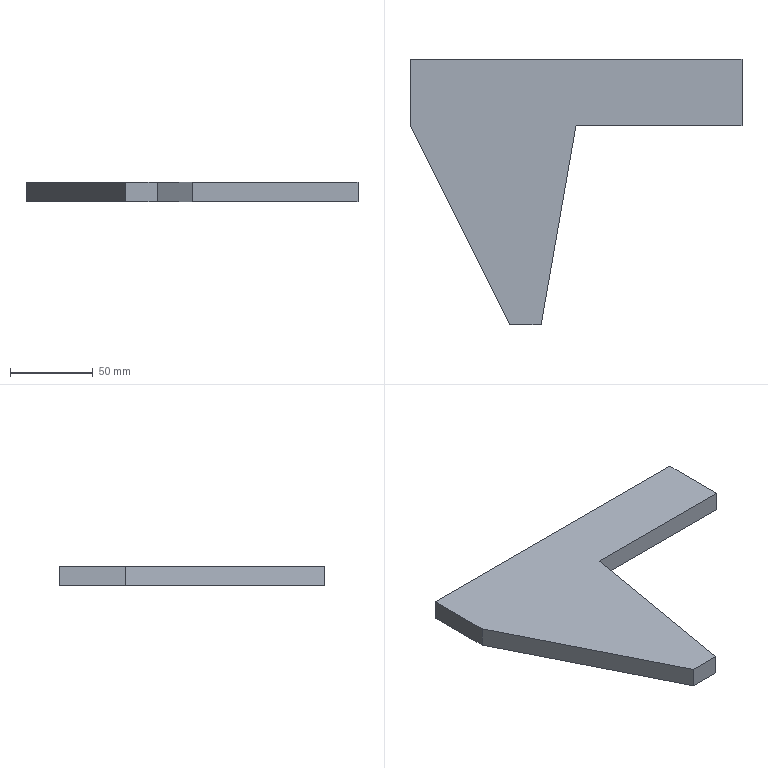Part | SolidWorks | features Extrusion 1, ICE 1 | 1 solid | 9 faces | box 200 x 160 x 12 mm | volume 181680 mm3 | plane 9
STEP:
#1=CARTESIAN_POINT('',(-100.,80.,0.));
#2=VERTEX_POINT('',#1);
#3=CARTESIAN_POINT('',(-100.,40.,0.));
#4=VERTEX_POINT('',#3);
#5=CARTESIAN_POINT('',(-100.,80.,0.));
#6=DIRECTION('',(0.,-1.,0.));
#7=VECTOR('',#6,1000.);
#8=LINE('',#5,#7);
#9=EDGE_CURVE('',#2,#4,#8,.T.);
#10=ORIENTED_EDGE('',*,*,#9,.T.);
#11=CARTESIAN_POINT('',(-100.,40.,12.));
#12=VERTEX_POINT('',#11);
#13=CARTESIAN_POINT('',(-100.,40.,0.));
#14=DIRECTION('',(0.,0.,1.));
#15=VECTOR('',#14,1000.);
#16=LINE('',#13,#15);
#17=EDGE_CURVE('',#4,#12,#16,.T.);
#18=ORIENTED_EDGE('',*,*,#17,.T.);
#19=CARTESIAN_POINT('',(-100.,80.,12.));
#20=VERTEX_POINT('',#19);
#21=CARTESIAN_POINT('',(-100.,80.,12.));
#22=DIRECTION('',(0.,-1.,0.));
#23=VECTOR('',#22,1000.);
#24=LINE('',#21,#23);
#25=EDGE_CURVE('',#20,#12,#24,.T.);
#26=ORIENTED_EDGE('',*,*,#25,.F.);
#27=CARTESIAN_POINT('',(-100.,80.,12.));
#28=DIRECTION('',(0.,0.,-1.));
#29=VECTOR('',#28,1000.);
#30=LINE('',#27,#29);
#31=EDGE_CURVE('',#20,#2,#30,.T.);
#32=ORIENTED_EDGE('',*,*,#31,.T.);
#33=EDGE_LOOP('',(#10,#18,#26,#32));
#34=FACE_OUTER_BOUND('',#33,.T.);
#35=CARTESIAN_POINT('',(-100.,80.,12.));
#36=DIRECTION('',(1.,0.,0.));
#37=DIRECTION('',(0.,1.,0.));
#38=AXIS2_PLACEMENT_3D('',#35,#36,#37);
#39=PLANE('',#38);
#40=ADVANCED_FACE('',(#34),#39,.F.);
#41=CARTESIAN_POINT('',(-40.,-80.,12.));
#42=VERTEX_POINT('',#41);
#43=CARTESIAN_POINT('',(-21.,-80.,12.));
#44=VERTEX_POINT('',#43);
#45=CARTESIAN_POINT('',(100.,-80.,12.));
#46=DIRECTION('',(1.,0.,0.));
#47=VECTOR('',#46,1000.);
#48=LINE('',#45,#47);
#49=EDGE_CURVE('',#42,#44,#48,.T.);
#50=ORIENTED_EDGE('',*,*,#49,.F.);
#51=CARTESIAN_POINT('',(-40.,-80.,0.));
#52=VERTEX_POINT('',#51);
#53=CARTESIAN_POINT('',(-40.,-80.,0.));
#54=DIRECTION('',(0.,0.,1.));
#55=VECTOR('',#54,1000.);
#56=LINE('',#53,#55);
#57=EDGE_CURVE('',#52,#42,#56,.T.);
#58=ORIENTED_EDGE('',*,*,#57,.F.);
#59=CARTESIAN_POINT('',(-21.,-80.,0.));
#60=VERTEX_POINT('',#59);
#61=CARTESIAN_POINT('',(100.,-80.,0.));
#62=DIRECTION('',(1.,0.,0.));
#63=VECTOR('',#62,1000.);
#64=LINE('',#61,#63);
#65=EDGE_CURVE('',#52,#60,#64,.T.);
#66=ORIENTED_EDGE('',*,*,#65,.T.);
#67=CARTESIAN_POINT('',(-21.,-80.,0.));
#68=DIRECTION('',(0.,0.,1.));
#69=VECTOR('',#68,1000.);
#70=LINE('',#67,#69);
#71=EDGE_CURVE('',#60,#44,#70,.T.);
#72=ORIENTED_EDGE('',*,*,#71,.T.);
#73=EDGE_LOOP('',(#50,#58,#66,#72));
#74=FACE_OUTER_BOUND('',#73,.T.);
#75=CARTESIAN_POINT('',(100.,-80.,12.));
#76=DIRECTION('',(0.,1.,0.));
#77=DIRECTION('',(-1.,0.,0.));
#78=AXIS2_PLACEMENT_3D('',#75,#76,#77);
#79=PLANE('',#78);
#80=ADVANCED_FACE('',(#74),#79,.F.);
#81=CARTESIAN_POINT('',(100.,40.,12.));
#82=VERTEX_POINT('',#81);
#83=CARTESIAN_POINT('',(100.,80.,12.));
#84=VERTEX_POINT('',#83);
#85=CARTESIAN_POINT('',(100.,80.,12.));
#86=DIRECTION('',(0.,1.,0.));
#87=VECTOR('',#86,1000.);
#88=LINE('',#85,#87);
#89=EDGE_CURVE('',#82,#84,#88,.T.);
#90=ORIENTED_EDGE('',*,*,#89,.F.);
#91=CARTESIAN_POINT('',(100.,40.,0.));
#92=VERTEX_POINT('',#91);
#93=CARTESIAN_POINT('',(100.,40.,0.));
#94=DIRECTION('',(0.,0.,1.));
#95=VECTOR('',#94,1000.);
#96=LINE('',#93,#95);
#97=EDGE_CURVE('',#92,#82,#96,.T.);
#98=ORIENTED_EDGE('',*,*,#97,.F.);
#99=CARTESIAN_POINT('',(100.,80.,0.));
#100=VERTEX_POINT('',#99);
#101=CARTESIAN_POINT('',(100.,80.,0.));
#102=DIRECTION('',(0.,1.,0.));
#103=VECTOR('',#102,1000.);
#104=LINE('',#101,#103);
#105=EDGE_CURVE('',#92,#100,#104,.T.);
#106=ORIENTED_EDGE('',*,*,#105,.T.);
#107=CARTESIAN_POINT('',(100.,80.,12.));
#108=DIRECTION('',(0.,0.,-1.));
#109=VECTOR('',#108,1000.);
#110=LINE('',#107,#109);
#111=EDGE_CURVE('',#84,#100,#110,.T.);
#112=ORIENTED_EDGE('',*,*,#111,.F.);
#113=EDGE_LOOP('',(#90,#98,#106,#112));
#114=FACE_OUTER_BOUND('',#113,.T.);
#115=CARTESIAN_POINT('',(100.,80.,12.));
#116=DIRECTION('',(-1.,0.,0.));
#117=DIRECTION('',(0.,-1.,0.));
#118=AXIS2_PLACEMENT_3D('',#115,#116,#117);
#119=PLANE('',#118);
#120=ADVANCED_FACE('',(#114),#119,.F.);
#121=CARTESIAN_POINT('',(100.,80.,0.));
#122=DIRECTION('',(-1.,0.,0.));
#123=VECTOR('',#122,1000.);
#124=LINE('',#121,#123);
#125=EDGE_CURVE('',#100,#2,#124,.T.);
#126=ORIENTED_EDGE('',*,*,#125,.T.);
#127=ORIENTED_EDGE('',*,*,#31,.F.);
#128=CARTESIAN_POINT('',(100.,80.,12.));
#129=DIRECTION('',(-1.,0.,0.));
#130=VECTOR('',#129,1000.);
#131=LINE('',#128,#130);
#132=EDGE_CURVE('',#84,#20,#131,.T.);
#133=ORIENTED_EDGE('',*,*,#132,.F.);
#134=ORIENTED_EDGE('',*,*,#111,.T.);
#135=EDGE_LOOP('',(#126,#127,#133,#134));
#136=FACE_OUTER_BOUND('',#135,.T.);
#137=CARTESIAN_POINT('',(100.,80.,12.));
#138=DIRECTION('',(0.,-1.,0.));
#139=DIRECTION('',(1.,0.,0.));
#140=AXIS2_PLACEMENT_3D('',#137,#138,#139);
#141=PLANE('',#140);
#142=ADVANCED_FACE('',(#136),#141,.F.);
#143=ORIENTED_EDGE('',*,*,#25,.T.);
#144=CARTESIAN_POINT('',(-100.,40.,12.));
#145=DIRECTION('',(-0.4472,0.8944,0.));
#146=VECTOR('',#145,1000.);
#147=LINE('',#144,#146);
#148=EDGE_CURVE('',#42,#12,#147,.T.);
#149=ORIENTED_EDGE('',*,*,#148,.F.);
#150=ORIENTED_EDGE('',*,*,#49,.T.);
#151=CARTESIAN_POINT('',(0.,40.,12.));
#152=VERTEX_POINT('',#151);
#153=CARTESIAN_POINT('',(-21.,-80.,12.));
#154=DIRECTION('',(-0.1724,-0.985,0.));
#155=VECTOR('',#154,1000.);
#156=LINE('',#153,#155);
#157=EDGE_CURVE('',#152,#44,#156,.T.);
#158=ORIENTED_EDGE('',*,*,#157,.F.);
#159=CARTESIAN_POINT('',(0.,40.,12.));
#160=DIRECTION('',(-1.,0.,0.));
#161=VECTOR('',#160,1000.);
#162=LINE('',#159,#161);
#163=EDGE_CURVE('',#82,#152,#162,.T.);
#164=ORIENTED_EDGE('',*,*,#163,.F.);
#165=ORIENTED_EDGE('',*,*,#89,.T.);
#166=ORIENTED_EDGE('',*,*,#132,.T.);
#167=EDGE_LOOP('',(#143,#149,#150,#158,#164,#165,#166));
#168=FACE_OUTER_BOUND('',#167,.T.);
#169=CARTESIAN_POINT('',(0.,0.,12.));
#170=DIRECTION('',(0.,0.,-1.));
#171=DIRECTION('',(-1.,0.,0.));
#172=AXIS2_PLACEMENT_3D('',#169,#170,#171);
#173=PLANE('',#172);
#174=ADVANCED_FACE('',(#168),#173,.F.);
#175=CARTESIAN_POINT('',(-100.,40.,0.));
#176=DIRECTION('',(-0.4472,0.8944,0.));
#177=VECTOR('',#176,1000.);
#178=LINE('',#175,#177);
#179=EDGE_CURVE('',#52,#4,#178,.T.);
#180=ORIENTED_EDGE('',*,*,#179,.T.);
#181=ORIENTED_EDGE('',*,*,#9,.F.);
#182=ORIENTED_EDGE('',*,*,#125,.F.);
#183=ORIENTED_EDGE('',*,*,#105,.F.);
#184=CARTESIAN_POINT('',(0.,40.,0.));
#185=VERTEX_POINT('',#184);
#186=CARTESIAN_POINT('',(0.,40.,0.));
#187=DIRECTION('',(-1.,0.,0.));
#188=VECTOR('',#187,1000.);
#189=LINE('',#186,#188);
#190=EDGE_CURVE('',#92,#185,#189,.T.);
#191=ORIENTED_EDGE('',*,*,#190,.T.);
#192=CARTESIAN_POINT('',(-21.,-80.,0.));
#193=DIRECTION('',(-0.1724,-0.985,0.));
#194=VECTOR('',#193,1000.);
#195=LINE('',#192,#194);
#196=EDGE_CURVE('',#185,#60,#195,.T.);
#197=ORIENTED_EDGE('',*,*,#196,.T.);
#198=ORIENTED_EDGE('',*,*,#65,.F.);
#199=EDGE_LOOP('',(#180,#181,#182,#183,#191,#197,#198));
#200=FACE_OUTER_BOUND('',#199,.T.);
#201=CARTESIAN_POINT('',(0.,0.,0.));
#202=DIRECTION('',(0.,0.,-1.));
#203=DIRECTION('',(-1.,0.,0.));
#204=AXIS2_PLACEMENT_3D('',#201,#202,#203);
#205=PLANE('',#204);
#206=ADVANCED_FACE('',(#200),#205,.T.);
#207=ORIENTED_EDGE('',*,*,#157,.T.);
#208=ORIENTED_EDGE('',*,*,#71,.F.);
#209=ORIENTED_EDGE('',*,*,#196,.F.);
#210=CARTESIAN_POINT('',(0.,40.,0.));
#211=DIRECTION('',(0.,0.,1.));
#212=VECTOR('',#211,1000.);
#213=LINE('',#210,#212);
#214=EDGE_CURVE('',#185,#152,#213,.T.);
#215=ORIENTED_EDGE('',*,*,#214,.T.);
#216=EDGE_LOOP('',(#207,#208,#209,#215));
#217=FACE_OUTER_BOUND('',#216,.T.);
#218=CARTESIAN_POINT('',(-21.,-80.,0.));
#219=DIRECTION('',(-0.985,0.1724,0.));
#220=DIRECTION('',(-0.1724,-0.985,0.));
#221=AXIS2_PLACEMENT_3D('',#218,#219,#220);
#222=PLANE('',#221);
#223=ADVANCED_FACE('',(#217),#222,.F.);
#224=ORIENTED_EDGE('',*,*,#163,.T.);
#225=ORIENTED_EDGE('',*,*,#214,.F.);
#226=ORIENTED_EDGE('',*,*,#190,.F.);
#227=ORIENTED_EDGE('',*,*,#97,.T.);
#228=EDGE_LOOP('',(#224,#225,#226,#227));
#229=FACE_OUTER_BOUND('',#228,.T.);
#230=CARTESIAN_POINT('',(0.,40.,0.));
#231=DIRECTION('',(0.,1.,0.));
#232=DIRECTION('',(0.,0.,1.));
#233=AXIS2_PLACEMENT_3D('',#230,#231,#232);
#234=PLANE('',#233);
#235=ADVANCED_FACE('',(#229),#234,.F.);
#236=ORIENTED_EDGE('',*,*,#148,.T.);
#237=ORIENTED_EDGE('',*,*,#17,.F.);
#238=ORIENTED_EDGE('',*,*,#179,.F.);
#239=ORIENTED_EDGE('',*,*,#57,.T.);
#240=EDGE_LOOP('',(#236,#237,#238,#239));
#241=FACE_OUTER_BOUND('',#240,.T.);
#242=CARTESIAN_POINT('',(-100.,40.,0.));
#243=DIRECTION('',(0.8944,0.4472,0.));
#244=DIRECTION('',(-0.4472,0.8944,0.));
#245=AXIS2_PLACEMENT_3D('',#242,#243,#244);
#246=PLANE('',#245);
#247=ADVANCED_FACE('',(#241),#246,.F.);
#248=CLOSED_SHELL('',(#40,#80,#120,#142,#174,#206,#223,#235,#247));
#249=MANIFOLD_SOLID_BREP('',#248);
#250=CARTESIAN_POINT('',(0.,0.,0.));
#251=DIRECTION('',(0.,0.,1.));
#252=DIRECTION('',(1.,0.,0.));
#253=AXIS2_PLACEMENT_3D('',#250,#251,#252);
#254=(LENGTH_UNIT()NAMED_UNIT(*)SI_UNIT(.MILLI.,.METRE.));
#255=UNCERTAINTY_MEASURE_WITH_UNIT(LENGTH_MEASURE(0.00001),#254,'','');
#256=(NAMED_UNIT(*)PLANE_ANGLE_UNIT()SI_UNIT($,.RADIAN.));
#257=(NAMED_UNIT(*)SI_UNIT($,.STERADIAN.)SOLID_ANGLE_UNIT());
#258=(GEOMETRIC_REPRESENTATION_CONTEXT(3)GLOBAL_UNCERTAINTY_ASSIGNED_CONTEXT((#255))GLOBAL_UNIT_ASSIGNED_CONTEXT((#254,#256,#257))REPRESENTATION_CONTEXT('',''));
#259=ADVANCED_BREP_SHAPE_REPRESENTATION('',(#249,#253),#258);